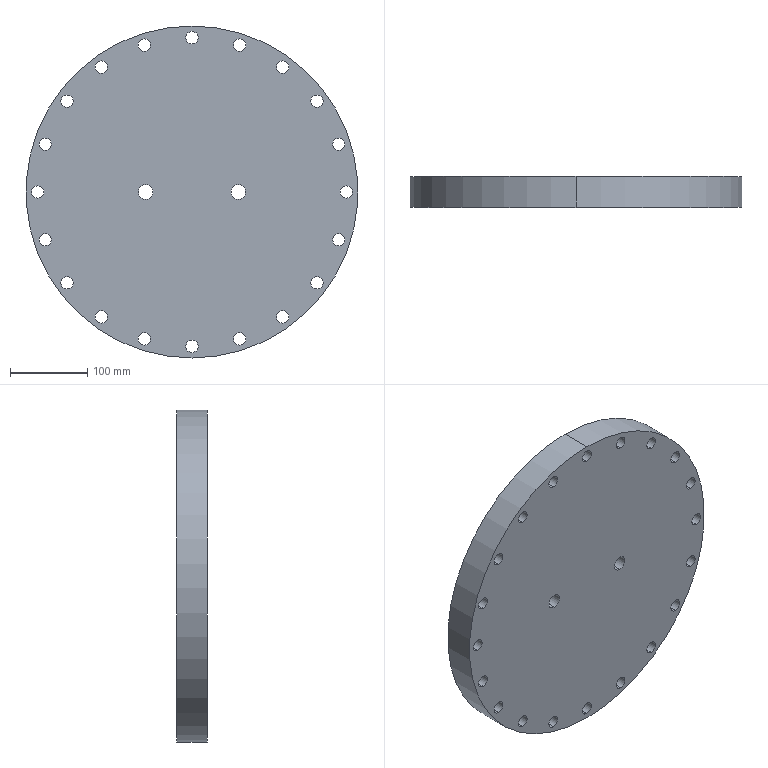Part | SolidWorks | features HoleWzd 2, Extrusion 1 | 1 solid | 48 faces | box 430 x 40 x 430 mm | volume 5625273 mm3 | cylinder 46 | plane 2 | commonest cylinder face diameters 16 x40 19 x4 430 x2